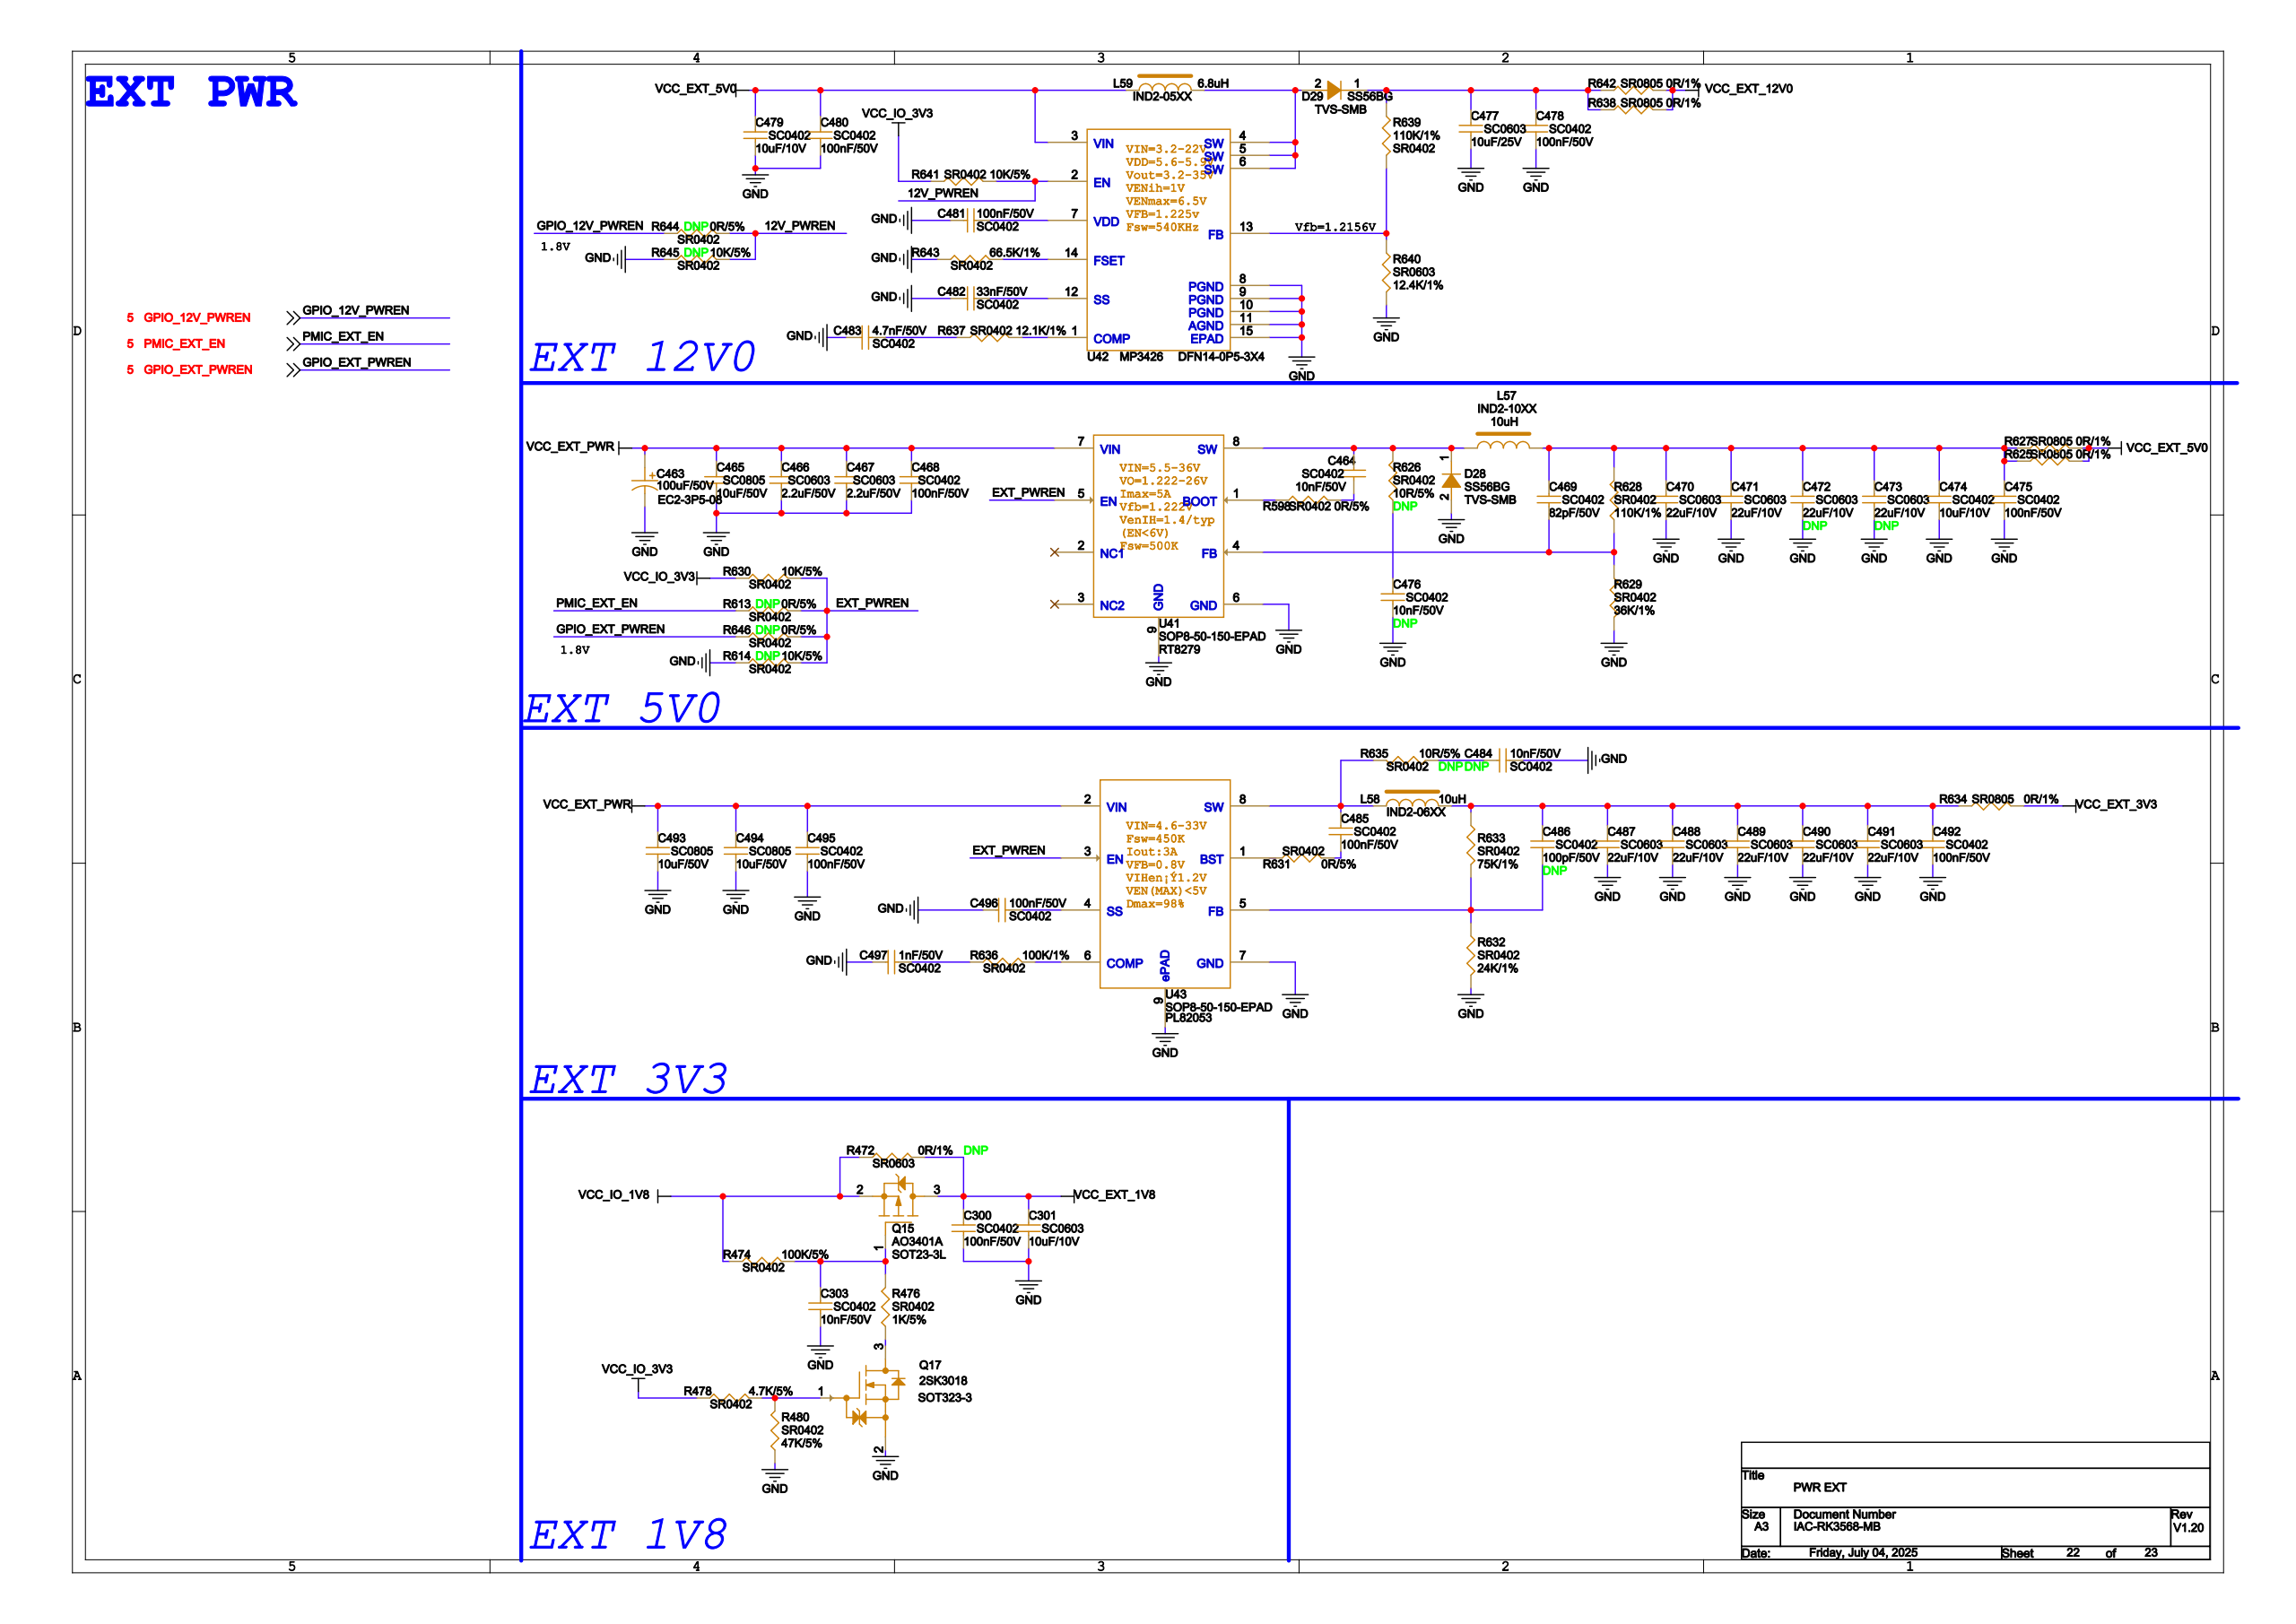Circuit board | Cadence Allegro | 1138 parts | 722 nets | one sheet of the schematic
Parts on this sheet (reference | value | footprint):
C300 | 100nF/50V | SC0402
C301 | 10uF/10V | SC0603
C303 | 10nF/50V | SC0402
C464 | 10nF/50V | SC0402
C465 | 10uF/50V | SC0805
C466 | 2.2uF/50V | SC0603
C467 | 2.2uF/50V | SC0603
C468 | 100nF/50V | SC0402
C469 | 82pF/50V | SC0402
C470 | 22uF/10V | SC0603
C471 | 22uF/10V | SC0603
C472 | 22uF/10V | SC0603
C473 | 22uF/10V | SC0603
C474 | 10uF/10V | SC0402
C475 | 100nF/50V | SC0402
C476 | 10nF/50V | SC0402
C477 | 10uF/25V | SC0603
C478 | 100nF/50V | SC0402
C479 | 10uF/10V | SC0402
C480 | 100nF/50V | SC0402
C481 | 100nF/50V | SC0402
C482 | 33nF/50V | SC0402
C483 | 4.7nF/50V | SC0402
C484 | 10nF/50V | SC0402
C485 | 100nF/50V | SC0402
C486 | 100pF/50V | SC0402
C487 | 22uF/10V | SC0603
C488 | 22uF/10V | SC0603
C489 | 22uF/10V | SC0603
C490 | 22uF/10V | SC0603
C491 | 22uF/10V | SC0603
C492 | 100nF/50V | SC0402
C493 | 10uF/50V | SC0805
C494 | 10uF/50V | SC0805
C495 | 100nF/50V | SC0402
C496 | 100nF/50V | SC0402
C497 | 1nF/50V | SC0402
D28 | SS56BG | TVS-SMB
D29 | SS56BG | TVS-SMB
L57 | 10uH | IND2-10XX
L58 | 10uH | IND2-06XX
L59 | 6.8uH | IND2-05XX
Q15 | AO3401A | SOT23-3L
Q17 | 2SK3018 | SOT323-3
R472 | 0R/1% | SR0603
R474 | 100K/5% | SR0402
R476 | 1K/5% | SR0402
R478 | 4.7K/5% | SR0402
R480 | 47K/5% | SR0402
R613 | 0R/5% | SR0402
R614 | 10K/5% | SR0402
R626 | 10R/5% | SR0402
R628 | 110K/1% | SR0402
R629 | 36K/1% | SR0402
R630 | 10K/5% | SR0402
R631 | 0R/5% | SR0402
R632 | 24K/1% | SR0402
R633 | 75K/1% | SR0402
R634 | 0R/1% | SR0805
R635 | 10R/5% | SR0402
R636 | 100K/1% | SR0402
R637 | 12.1K/1% | SR0402
R638 | 0R/1% | SR0805
R639 | 110K/1% | SR0402
R640 | 12.4K/1% | SR0603
R641 | 10K/5% | SR0402
R642 | 0R/1% | SR0805
R643 | 66.5K/1% | SR0402
R644 | 0R/5% | SR0402
R645 | 10K/5% | SR0402
R646 | 0R/5% | SR0402
U41 | RT8279 | SOP8-50-150-EPAD
U42 | MP3426 | DFN14-0P5-3X4
U43 | PL82053 | SOP8-50-150-EPAD
Nets of these parts (net: part-pin ...):
VCC_EXT_5V0: C479-1 C480-1 L59-1 U42-3
VCC_EXT_3V3: R634-2
GND: C300-2 C301-2 C303-2 C465-2 C466-2 C467-2 C468-2 C470-2 C471-2 C472-2 C473-2 C474-2 C475-2 C476-2 C477-2 C478-2 C479-2 C480-2 C481-2 C482-2 C483-1 C484-2 C487-2 C488-2 C489-2 C490-2 C491-2 C492-2 C493-2 C494-2 C495-2 C496-1 C497-1 D28-2 Q17-2 R480-1 R614-1 R629-2 R632-2 R640-2 R643-1 R645-1 U41-6 U41-9 U42-8 U42-9 U42-10 U42-11 U42-15 U43-7 U43-9
N16107320: C464-1 D28-1 L57-1 R626-2 U41-8
N16416307: D29-2 L59-2 U42-4 U42-5 U42-6
N16416315: C477-1 C478-1 D29-1 R638-1 R639-1 R642-1
VCC_EXT_PWR: C465-1 C466-1 C467-1 C468-1 C493-1 C494-1 C495-1 U41-7 U43-2
N16107328: C469-1 C470-1 C471-1 C472-1 C473-1 C474-1 C475-1 L57-2 R628-2
N16107364: C469-2 R628-1 R629-1 U41-4
N16416275: C482-1 U42-12
N16107520: C476-1 R626-1
N16412370: C484-1 R635-1
N16411930: C485-1 L58-1 R635-2 U43-8
N16416219: R639-2 R640-1 U42-13
N16412180: C486-2 R632-1 R633-2 U43-5
N16412184: C486-1 C487-1 C488-1 C489-1 C490-1 C491-1 C492-1 L58-2 R633-1 R634-1
N16416295: C483-2 R637-1
N16416291: R637-2 U42-1
N16416283: R643-2 U42-14
N16107360: U41-1
EXT_PWREN: R613-2 R614-2 R630-2 R646-2 U41-5 U43-3
12V_PWREN: R641-2 R644-2 R645-2 U42-2
N16416299: C481-1 U42-7
N16411944: R631-1 U43-1
N16412476: R636-2 U43-6
N16411908: C496-2 U43-4
VCC_EXT_1V8: C300-1 C301-1 Q15-3 R472-2
N4114718: C303-1 Q15-1 R474-2 R476-2
VCC_IO_1V8: Q15-2 R472-1 R474-1
N4114740: Q17-3 R476-1
N4114840: Q17-1 R478-2 R480-2
VCC_IO_3V3: R478-1 R630-1 R641-1
N16411896: C497-2 R636-1
N16107308: C464-2
VCC_EXT_12V0: R638-2 R642-2
GPIO_12V_PWREN: R644-1
GPIO_EXT_PWREN: R646-1
PMIC_EXT_EN: R613-1
N16411940: C485-2 R631-2